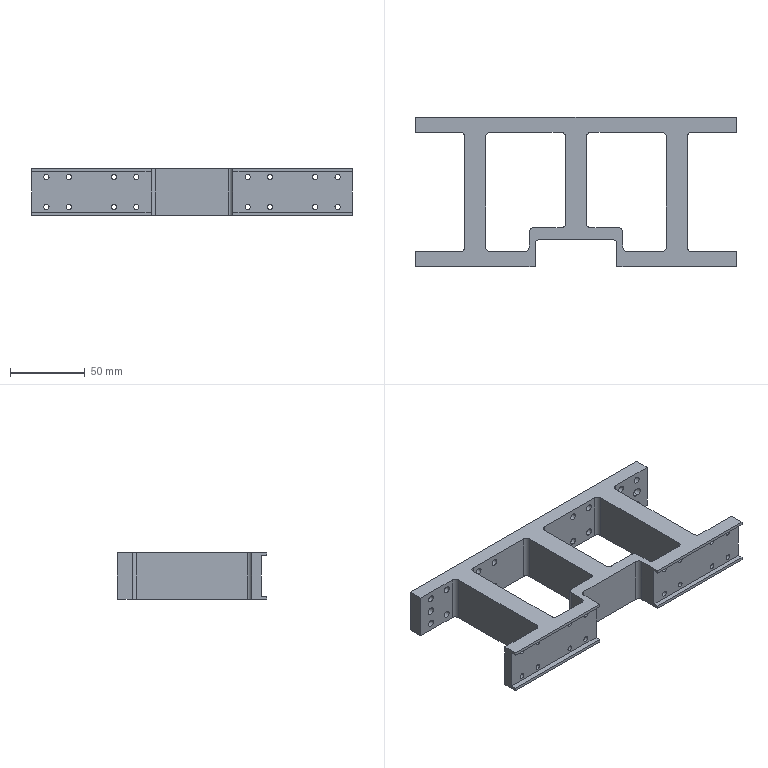Part | 1 solid | 127 faces | box 215 x 100 x 31 mm | volume 212754 mm3 | cylinder 87 | plane 40 | commonest cylinder face diameters 3.5 x32 4.5 x32 6 x18 5 x5